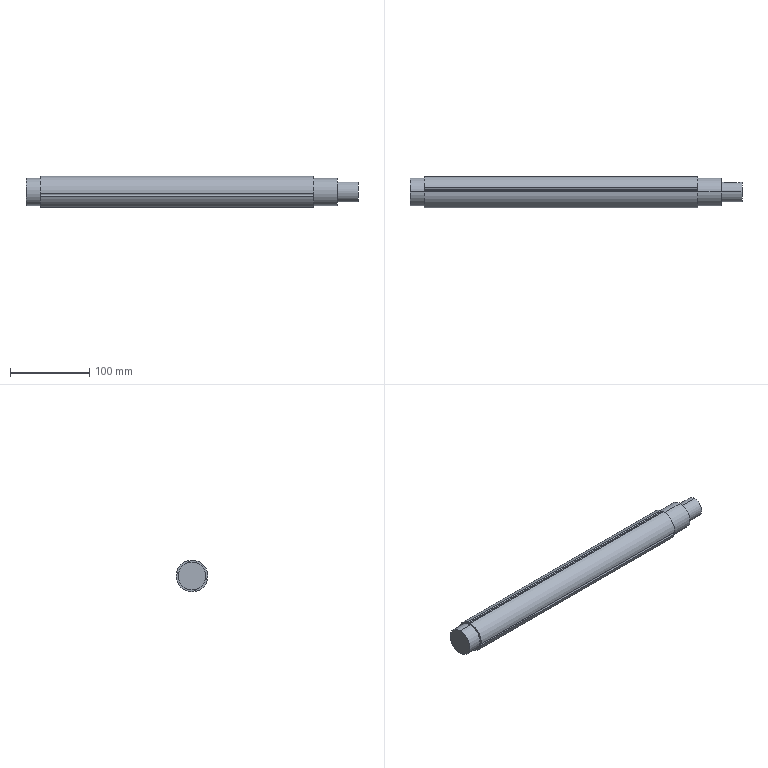Part | SolidWorks | features ICE 6, RefAxis 3, 3DProfileFeature 1, LockFeature 1, Revolution 1 | 1 solid | 26 faces | box 419 x 40 x 40 mm | volume 488497 mm3 | cylinder 18 | plane 8 | commonest cylinder face diameters 4.38 x5 40 x5 35 x4 8 x2 25 x2
STEP:
#1=CARTESIAN_POINT('',(193.5,11.843,-4.));
#2=VERTEX_POINT('',#1);
#3=CARTESIAN_POINT('',(193.5,11.843,4.));
#4=VERTEX_POINT('',#3);
#5=CARTESIAN_POINT('',(193.5,11.843,-4.));
#6=CARTESIAN_POINT('',(193.234,11.843,-4.));
#7=CARTESIAN_POINT('',(192.973,11.852,-3.974));
#8=CARTESIAN_POINT('',(192.459,11.886,-3.871));
#9=CARTESIAN_POINT('',(192.204,11.911,-3.793));
#10=CARTESIAN_POINT('',(191.721,11.973,-3.592));
#11=CARTESIAN_POINT('',(191.492,12.01,-3.469));
#12=CARTESIAN_POINT('',(191.059,12.09,-3.179));
#13=CARTESIAN_POINT('',(190.855,12.133,-3.012));
#14=CARTESIAN_POINT('',(190.489,12.218,-2.646));
#15=CARTESIAN_POINT('',(190.324,12.26,-2.445));
#16=CARTESIAN_POINT('',(190.031,12.34,-2.009));
#17=CARTESIAN_POINT('',(189.908,12.375,-1.779));
#18=CARTESIAN_POINT('',(189.708,12.435,-1.299));
#19=CARTESIAN_POINT('',(189.63,12.459,-1.045));
#20=CARTESIAN_POINT('',(189.526,12.492,-0.5276));
#21=CARTESIAN_POINT('',(189.5,12.5,-0.2669));
#22=CARTESIAN_POINT('',(189.5,12.5,0.2587));
#23=CARTESIAN_POINT('',(189.526,12.492,0.5256));
#24=CARTESIAN_POINT('',(189.629,12.459,1.04));
#25=CARTESIAN_POINT('',(189.705,12.436,1.29));
#26=CARTESIAN_POINT('',(189.907,12.375,1.777));
#27=CARTESIAN_POINT('',(190.031,12.34,2.008));
#28=CARTESIAN_POINT('',(190.32,12.262,2.44));
#29=CARTESIAN_POINT('',(190.487,12.219,2.643));
#30=CARTESIAN_POINT('',(190.855,12.133,3.012));
#31=CARTESIAN_POINT('',(191.055,12.091,3.176));
#32=CARTESIAN_POINT('',(191.487,12.011,3.466));
#33=CARTESIAN_POINT('',(191.72,11.973,3.592));
#34=CARTESIAN_POINT('',(192.202,11.911,3.792));
#35=CARTESIAN_POINT('',(192.451,11.886,3.869));
#36=CARTESIAN_POINT('',(192.968,11.852,3.973));
#37=CARTESIAN_POINT('',(193.234,11.843,4.));
#38=CARTESIAN_POINT('',(193.5,11.843,4.));
#39=B_SPLINE_CURVE_WITH_KNOTS('',3,(#5,#6,#7,#8,#9,#10,#11,#12,#13,#14,#15,#16,#17,#18,#19,#20,#21,#22,#23,#24,#25,#26,#27,#28,#29,#30,#31,#32,#33,#34,#35,#36,#37,#38),.UNSPECIFIED.,.F.,.F.,(4,2,2,2,2,2,2,2,2,2,2,2,2,2,2,2,4),(0.,0.0007865,0.001573,0.00236,0.003146,0.003933,0.004719,0.005506,0.006292,0.007079,0.007865,0.008652,0.009438,0.01022,0.01101,0.0118,0.01258),.UNSPECIFIED.);
#40=EDGE_CURVE('',#2,#4,#39,.T.);
#41=ORIENTED_EDGE('',*,*,#40,.F.);
#42=CARTESIAN_POINT('',(208.5,11.843,-4.));
#43=VERTEX_POINT('',#42);
#44=CARTESIAN_POINT('',(187.5,11.843,-4.));
#45=DIRECTION('',(-1.,0.,0.));
#46=VECTOR('',#45,1000.);
#47=LINE('',#44,#46);
#48=EDGE_CURVE('',#43,#2,#47,.T.);
#49=ORIENTED_EDGE('',*,*,#48,.F.);
#50=CARTESIAN_POINT('',(208.5,11.843,4.));
#51=VERTEX_POINT('',#50);
#52=CARTESIAN_POINT('',(208.5,11.843,4.));
#53=CARTESIAN_POINT('',(208.766,11.843,4.));
#54=CARTESIAN_POINT('',(209.027,11.852,3.974));
#55=CARTESIAN_POINT('',(209.541,11.886,3.871));
#56=CARTESIAN_POINT('',(209.796,11.911,3.793));
#57=CARTESIAN_POINT('',(210.279,11.973,3.592));
#58=CARTESIAN_POINT('',(210.508,12.01,3.469));
#59=CARTESIAN_POINT('',(210.941,12.09,3.179));
#60=CARTESIAN_POINT('',(211.145,12.133,3.012));
#61=CARTESIAN_POINT('',(211.511,12.218,2.646));
#62=CARTESIAN_POINT('',(211.676,12.26,2.445));
#63=CARTESIAN_POINT('',(211.969,12.34,2.009));
#64=CARTESIAN_POINT('',(212.092,12.375,1.779));
#65=CARTESIAN_POINT('',(212.292,12.435,1.299));
#66=CARTESIAN_POINT('',(212.37,12.459,1.045));
#67=CARTESIAN_POINT('',(212.474,12.492,0.5276));
#68=CARTESIAN_POINT('',(212.5,12.5,0.2669));
#69=CARTESIAN_POINT('',(212.5,12.5,-0.2587));
#70=CARTESIAN_POINT('',(212.474,12.492,-0.5256));
#71=CARTESIAN_POINT('',(212.371,12.459,-1.04));
#72=CARTESIAN_POINT('',(212.295,12.436,-1.29));
#73=CARTESIAN_POINT('',(212.093,12.375,-1.777));
#74=CARTESIAN_POINT('',(211.969,12.34,-2.008));
#75=CARTESIAN_POINT('',(211.68,12.262,-2.44));
#76=CARTESIAN_POINT('',(211.513,12.219,-2.643));
#77=CARTESIAN_POINT('',(211.145,12.133,-3.012));
#78=CARTESIAN_POINT('',(210.945,12.091,-3.176));
#79=CARTESIAN_POINT('',(210.513,12.011,-3.466));
#80=CARTESIAN_POINT('',(210.28,11.973,-3.592));
#81=CARTESIAN_POINT('',(209.798,11.911,-3.792));
#82=CARTESIAN_POINT('',(209.549,11.886,-3.869));
#83=CARTESIAN_POINT('',(209.032,11.852,-3.973));
#84=CARTESIAN_POINT('',(208.766,11.843,-4.));
#85=CARTESIAN_POINT('',(208.5,11.843,-4.));
#86=B_SPLINE_CURVE_WITH_KNOTS('',3,(#52,#53,#54,#55,#56,#57,#58,#59,#60,#61,#62,#63,#64,#65,#66,#67,#68,#69,#70,#71,#72,#73,#74,#75,#76,#77,#78,#79,#80,#81,#82,#83,#84,#85),.UNSPECIFIED.,.F.,.F.,(4,2,2,2,2,2,2,2,2,2,2,2,2,2,2,2,4),(0.,0.0007865,0.001573,0.00236,0.003146,0.003933,0.004719,0.005506,0.006292,0.007079,0.007865,0.008652,0.009438,0.01022,0.01101,0.0118,0.01258),.UNSPECIFIED.);
#87=EDGE_CURVE('',#51,#43,#86,.T.);
#88=ORIENTED_EDGE('',*,*,#87,.F.);
#89=CARTESIAN_POINT('',(187.5,11.843,4.));
#90=DIRECTION('',(1.,0.,0.));
#91=VECTOR('',#90,1000.);
#92=LINE('',#89,#91);
#93=EDGE_CURVE('',#4,#51,#92,.T.);
#94=ORIENTED_EDGE('',*,*,#93,.F.);
#95=EDGE_LOOP('',(#41,#49,#88,#94));
#96=FACE_BOUND('',#95,.T.);
#97=CARTESIAN_POINT('',(187.5,0.,-12.5));
#98=VERTEX_POINT('',#97);
#99=CARTESIAN_POINT('',(187.5,0.,12.5));
#100=VERTEX_POINT('',#99);
#101=CARTESIAN_POINT('',(187.5,0.,0.));
#102=DIRECTION('',(1.,0.,0.));
#103=DIRECTION('',(0.,0.,-1.));
#104=AXIS2_PLACEMENT_3D('',#101,#102,#103);
#105=CIRCLE('',#104,12.5);
#106=EDGE_CURVE('',#98,#100,#105,.T.);
#107=ORIENTED_EDGE('',*,*,#106,.T.);
#108=CARTESIAN_POINT('',(213.5,0.,12.5));
#109=VERTEX_POINT('',#108);
#110=CARTESIAN_POINT('',(187.5,0.,12.5));
#111=DIRECTION('',(1.,0.,0.));
#112=VECTOR('',#111,1000.);
#113=LINE('',#110,#112);
#114=EDGE_CURVE('',#100,#109,#113,.T.);
#115=ORIENTED_EDGE('',*,*,#114,.T.);
#116=CARTESIAN_POINT('',(213.5,0.,-12.5));
#117=VERTEX_POINT('',#116);
#118=CARTESIAN_POINT('',(213.5,0.,0.));
#119=DIRECTION('',(1.,0.,0.));
#120=DIRECTION('',(0.,0.,-1.));
#121=AXIS2_PLACEMENT_3D('',#118,#119,#120);
#122=CIRCLE('',#121,12.5);
#123=EDGE_CURVE('',#117,#109,#122,.T.);
#124=ORIENTED_EDGE('',*,*,#123,.F.);
#125=CARTESIAN_POINT('',(187.5,0.,-12.5));
#126=DIRECTION('',(1.,0.,0.));
#127=VECTOR('',#126,1000.);
#128=LINE('',#125,#127);
#129=EDGE_CURVE('',#98,#117,#128,.T.);
#130=ORIENTED_EDGE('',*,*,#129,.F.);
#131=EDGE_LOOP('',(#107,#115,#124,#130));
#132=FACE_OUTER_BOUND('',#131,.T.);
#133=CARTESIAN_POINT('',(187.5,0.,0.));
#134=DIRECTION('',(1.,0.,0.));
#135=DIRECTION('',(0.,0.,-1.));
#136=AXIS2_PLACEMENT_3D('',#133,#134,#135);
#137=CYLINDRICAL_SURFACE('',#136,12.5);
#138=ADVANCED_FACE('',(#96,#132),#137,.T.);
#139=CARTESIAN_POINT('',(157.5,0.,-17.5));
#140=VERTEX_POINT('',#139);
#141=CARTESIAN_POINT('',(157.5,0.,17.5));
#142=VERTEX_POINT('',#141);
#143=CARTESIAN_POINT('',(157.5,0.,0.));
#144=DIRECTION('',(1.,0.,0.));
#145=DIRECTION('',(0.,0.,-1.));
#146=AXIS2_PLACEMENT_3D('',#143,#144,#145);
#147=CIRCLE('',#146,17.5);
#148=EDGE_CURVE('',#140,#142,#147,.T.);
#149=ORIENTED_EDGE('',*,*,#148,.T.);
#150=CARTESIAN_POINT('',(187.5,0.,17.5));
#151=VERTEX_POINT('',#150);
#152=CARTESIAN_POINT('',(157.5,0.,17.5));
#153=DIRECTION('',(1.,0.,0.));
#154=VECTOR('',#153,1000.);
#155=LINE('',#152,#154);
#156=EDGE_CURVE('',#142,#151,#155,.T.);
#157=ORIENTED_EDGE('',*,*,#156,.T.);
#158=CARTESIAN_POINT('',(187.5,0.,-17.5));
#159=VERTEX_POINT('',#158);
#160=CARTESIAN_POINT('',(187.5,0.,0.));
#161=DIRECTION('',(1.,0.,0.));
#162=DIRECTION('',(0.,0.,-1.));
#163=AXIS2_PLACEMENT_3D('',#160,#161,#162);
#164=CIRCLE('',#163,17.5);
#165=EDGE_CURVE('',#159,#151,#164,.T.);
#166=ORIENTED_EDGE('',*,*,#165,.F.);
#167=CARTESIAN_POINT('',(157.5,0.,-17.5));
#168=DIRECTION('',(1.,0.,0.));
#169=VECTOR('',#168,1000.);
#170=LINE('',#167,#169);
#171=EDGE_CURVE('',#140,#159,#170,.T.);
#172=ORIENTED_EDGE('',*,*,#171,.F.);
#173=EDGE_LOOP('',(#149,#157,#166,#172));
#174=FACE_OUTER_BOUND('',#173,.T.);
#175=CARTESIAN_POINT('',(157.5,0.,0.));
#176=DIRECTION('',(1.,0.,0.));
#177=DIRECTION('',(0.,0.,-1.));
#178=AXIS2_PLACEMENT_3D('',#175,#176,#177);
#179=CYLINDRICAL_SURFACE('',#178,17.5);
#180=ADVANCED_FACE('',(#174),#179,.T.);
#181=CARTESIAN_POINT('',(-187.5,0.,17.5));
#182=VERTEX_POINT('',#181);
#183=CARTESIAN_POINT('',(-187.5,0.,-17.5));
#184=VERTEX_POINT('',#183);
#185=CARTESIAN_POINT('',(-187.5,0.,0.));
#186=DIRECTION('',(-1.,0.,0.));
#187=DIRECTION('',(0.,0.,1.));
#188=AXIS2_PLACEMENT_3D('',#185,#186,#187);
#189=CIRCLE('',#188,17.5);
#190=EDGE_CURVE('',#182,#184,#189,.T.);
#191=ORIENTED_EDGE('',*,*,#190,.T.);
#192=CARTESIAN_POINT('',(-205.5,0.,-17.5));
#193=VERTEX_POINT('',#192);
#194=CARTESIAN_POINT('',(-187.5,0.,-17.5));
#195=DIRECTION('',(-1.,0.,0.));
#196=VECTOR('',#195,1000.);
#197=LINE('',#194,#196);
#198=EDGE_CURVE('',#184,#193,#197,.T.);
#199=ORIENTED_EDGE('',*,*,#198,.T.);
#200=CARTESIAN_POINT('',(-205.5,0.,17.5));
#201=VERTEX_POINT('',#200);
#202=CARTESIAN_POINT('',(-205.5,0.,0.));
#203=DIRECTION('',(-1.,0.,0.));
#204=DIRECTION('',(0.,0.,1.));
#205=AXIS2_PLACEMENT_3D('',#202,#203,#204);
#206=CIRCLE('',#205,17.5);
#207=EDGE_CURVE('',#201,#193,#206,.T.);
#208=ORIENTED_EDGE('',*,*,#207,.F.);
#209=CARTESIAN_POINT('',(-187.5,0.,17.5));
#210=DIRECTION('',(-1.,0.,0.));
#211=VECTOR('',#210,1000.);
#212=LINE('',#209,#211);
#213=EDGE_CURVE('',#182,#201,#212,.T.);
#214=ORIENTED_EDGE('',*,*,#213,.F.);
#215=EDGE_LOOP('',(#191,#199,#208,#214));
#216=FACE_OUTER_BOUND('',#215,.T.);
#217=CARTESIAN_POINT('',(-187.5,0.,0.));
#218=DIRECTION('',(-1.,0.,0.));
#219=DIRECTION('',(0.,0.,1.));
#220=AXIS2_PLACEMENT_3D('',#217,#218,#219);
#221=CYLINDRICAL_SURFACE('',#220,17.5);
#222=ADVANCED_FACE('',(#216),#221,.T.);
#223=CARTESIAN_POINT('',(-187.5,5.203,19.311));
#224=VERTEX_POINT('',#223);
#225=CARTESIAN_POINT('',(-187.5,3.683,18.698));
#226=VERTEX_POINT('',#225);
#227=CARTESIAN_POINT('',(-187.5,3.683,20.888));
#228=DIRECTION('',(-1.,0.,0.));
#229=DIRECTION('',(0.,0.,1.));
#230=AXIS2_PLACEMENT_3D('',#227,#228,#229);
#231=CIRCLE('',#230,2.19);
#232=EDGE_CURVE('',#224,#226,#231,.T.);
#233=ORIENTED_EDGE('',*,*,#232,.T.);
#234=CARTESIAN_POINT('',(157.5,3.683,18.698));
#235=VERTEX_POINT('',#234);
#236=CARTESIAN_POINT('',(-205.5,3.683,18.698));
#237=DIRECTION('',(1.,0.,0.));
#238=VECTOR('',#237,1000.);
#239=LINE('',#236,#238);
#240=EDGE_CURVE('',#226,#235,#239,.T.);
#241=ORIENTED_EDGE('',*,*,#240,.T.);
#242=CARTESIAN_POINT('',(157.5,5.203,19.311));
#243=VERTEX_POINT('',#242);
#244=CARTESIAN_POINT('',(157.5,3.683,20.888));
#245=DIRECTION('',(1.,0.,0.));
#246=DIRECTION('',(0.,0.,-1.));
#247=AXIS2_PLACEMENT_3D('',#244,#245,#246);
#248=CIRCLE('',#247,2.19);
#249=EDGE_CURVE('',#235,#243,#248,.T.);
#250=ORIENTED_EDGE('',*,*,#249,.T.);
#251=CARTESIAN_POINT('',(-205.5,5.203,19.311));
#252=DIRECTION('',(1.,0.,0.));
#253=VECTOR('',#252,1000.);
#254=LINE('',#251,#253);
#255=EDGE_CURVE('',#224,#243,#254,.T.);
#256=ORIENTED_EDGE('',*,*,#255,.F.);
#257=EDGE_LOOP('',(#233,#241,#250,#256));
#258=FACE_OUTER_BOUND('',#257,.T.);
#259=CARTESIAN_POINT('',(-205.5,3.683,20.888));
#260=DIRECTION('',(1.,0.,0.));
#261=DIRECTION('',(0.,0.,-1.));
#262=AXIS2_PLACEMENT_3D('',#259,#260,#261);
#263=CYLINDRICAL_SURFACE('',#262,2.19);
#264=ADVANCED_FACE('',(#258),#263,.F.);
#265=CARTESIAN_POINT('',(157.5,0.,20.));
#266=VERTEX_POINT('',#265);
#267=CARTESIAN_POINT('',(157.5,-19.926,-1.715));
#268=VERTEX_POINT('',#267);
#269=CARTESIAN_POINT('',(157.5,0.,0.));
#270=DIRECTION('',(1.,0.,0.));
#271=DIRECTION('',(0.,0.,-1.));
#272=AXIS2_PLACEMENT_3D('',#269,#270,#271);
#273=CIRCLE('',#272,20.);
#274=EDGE_CURVE('',#266,#268,#273,.T.);
#275=ORIENTED_EDGE('',*,*,#274,.F.);
#276=CARTESIAN_POINT('',(-187.5,0.,20.));
#277=VERTEX_POINT('',#276);
#278=CARTESIAN_POINT('',(205.5,0.,20.));
#279=DIRECTION('',(-1.,0.,0.));
#280=VECTOR('',#279,1000.);
#281=LINE('',#278,#280);
#282=EDGE_CURVE('',#266,#277,#281,.T.);
#283=ORIENTED_EDGE('',*,*,#282,.T.);
#284=CARTESIAN_POINT('',(-187.5,-19.926,-1.715));
#285=VERTEX_POINT('',#284);
#286=CARTESIAN_POINT('',(-187.5,0.,0.));
#287=DIRECTION('',(-1.,0.,0.));
#288=DIRECTION('',(0.,0.,1.));
#289=AXIS2_PLACEMENT_3D('',#286,#287,#288);
#290=CIRCLE('',#289,20.);
#291=EDGE_CURVE('',#285,#277,#290,.T.);
#292=ORIENTED_EDGE('',*,*,#291,.F.);
#293=CARTESIAN_POINT('',(-205.5,-19.926,-1.715));
#294=DIRECTION('',(1.,0.,0.));
#295=VECTOR('',#294,1000.);
#296=LINE('',#293,#295);
#297=EDGE_CURVE('',#285,#268,#296,.T.);
#298=ORIENTED_EDGE('',*,*,#297,.T.);
#299=EDGE_LOOP('',(#275,#283,#292,#298));
#300=FACE_OUTER_BOUND('',#299,.T.);
#301=CARTESIAN_POINT('',(205.5,0.,0.));
#302=DIRECTION('',(-1.,0.,0.));
#303=DIRECTION('',(0.,0.,1.));
#304=AXIS2_PLACEMENT_3D('',#301,#302,#303);
#305=CYLINDRICAL_SURFACE('',#304,20.);
#306=ADVANCED_FACE('',(#300),#305,.T.);
#307=CARTESIAN_POINT('',(157.5,19.311,5.203));
#308=VERTEX_POINT('',#307);
#309=CARTESIAN_POINT('',(157.5,0.,0.));
#310=DIRECTION('',(1.,0.,0.));
#311=DIRECTION('',(0.,0.,-1.));
#312=AXIS2_PLACEMENT_3D('',#309,#310,#311);
#313=CIRCLE('',#312,20.);
#314=EDGE_CURVE('',#308,#243,#313,.T.);
#315=ORIENTED_EDGE('',*,*,#314,.F.);
#316=CARTESIAN_POINT('',(-187.5,19.311,5.203));
#317=VERTEX_POINT('',#316);
#318=CARTESIAN_POINT('',(-205.5,19.311,5.203));
#319=DIRECTION('',(1.,0.,0.));
#320=VECTOR('',#319,1000.);
#321=LINE('',#318,#320);
#322=EDGE_CURVE('',#317,#308,#321,.T.);
#323=ORIENTED_EDGE('',*,*,#322,.F.);
#324=CARTESIAN_POINT('',(-187.5,0.,0.));
#325=DIRECTION('',(-1.,0.,0.));
#326=DIRECTION('',(0.,0.,1.));
#327=AXIS2_PLACEMENT_3D('',#324,#325,#326);
#328=CIRCLE('',#327,20.);
#329=EDGE_CURVE('',#224,#317,#328,.T.);
#330=ORIENTED_EDGE('',*,*,#329,.F.);
#331=ORIENTED_EDGE('',*,*,#255,.T.);
#332=EDGE_LOOP('',(#315,#323,#330,#331));
#333=FACE_OUTER_BOUND('',#332,.T.);
#334=CARTESIAN_POINT('',(205.5,0.,0.));
#335=DIRECTION('',(-1.,0.,0.));
#336=DIRECTION('',(0.,0.,1.));
#337=AXIS2_PLACEMENT_3D('',#334,#335,#336);
#338=CYLINDRICAL_SURFACE('',#337,20.);
#339=ADVANCED_FACE('',(#333),#338,.T.);
#340=ORIENTED_EDGE('',*,*,#282,.F.);
#341=CARTESIAN_POINT('',(157.5,1.715,19.926));
#342=VERTEX_POINT('',#341);
#343=CARTESIAN_POINT('',(157.5,0.,0.));
#344=DIRECTION('',(1.,0.,0.));
#345=DIRECTION('',(0.,0.,-1.));
#346=AXIS2_PLACEMENT_3D('',#343,#344,#345);
#347=CIRCLE('',#346,20.);
#348=EDGE_CURVE('',#342,#266,#347,.T.);
#349=ORIENTED_EDGE('',*,*,#348,.F.);
#350=CARTESIAN_POINT('',(-187.5,1.715,19.926));
#351=VERTEX_POINT('',#350);
#352=CARTESIAN_POINT('',(-205.5,1.715,19.926));
#353=DIRECTION('',(1.,0.,0.));
#354=VECTOR('',#353,1000.);
#355=LINE('',#352,#354);
#356=EDGE_CURVE('',#351,#342,#355,.T.);
#357=ORIENTED_EDGE('',*,*,#356,.F.);
#358=CARTESIAN_POINT('',(-187.5,0.,0.));
#359=DIRECTION('',(-1.,0.,0.));
#360=DIRECTION('',(0.,0.,1.));
#361=AXIS2_PLACEMENT_3D('',#358,#359,#360);
#362=CIRCLE('',#361,20.);
#363=EDGE_CURVE('',#277,#351,#362,.T.);
#364=ORIENTED_EDGE('',*,*,#363,.F.);
#365=EDGE_LOOP('',(#340,#349,#357,#364));
#366=FACE_OUTER_BOUND('',#365,.T.);
#367=CARTESIAN_POINT('',(205.5,0.,0.));
#368=DIRECTION('',(-1.,0.,0.));
#369=DIRECTION('',(0.,0.,1.));
#370=AXIS2_PLACEMENT_3D('',#367,#368,#369);
#371=CYLINDRICAL_SURFACE('',#370,20.);
#372=ADVANCED_FACE('',(#366),#371,.T.);
#373=CARTESIAN_POINT('',(157.5,-1.715,-19.926));
#374=VERTEX_POINT('',#373);
#375=CARTESIAN_POINT('',(157.5,19.926,1.715));
#376=VERTEX_POINT('',#375);
#377=CARTESIAN_POINT('',(157.5,0.,0.));
#378=DIRECTION('',(1.,0.,0.));
#379=DIRECTION('',(0.,0.,-1.));
#380=AXIS2_PLACEMENT_3D('',#377,#378,#379);
#381=CIRCLE('',#380,20.);
#382=EDGE_CURVE('',#374,#376,#381,.T.);
#383=ORIENTED_EDGE('',*,*,#382,.F.);
#384=CARTESIAN_POINT('',(-187.5,-1.715,-19.926));
#385=VERTEX_POINT('',#384);
#386=CARTESIAN_POINT('',(-205.5,-1.715,-19.926));
#387=DIRECTION('',(1.,0.,0.));
#388=VECTOR('',#387,1000.);
#389=LINE('',#386,#388);
#390=EDGE_CURVE('',#385,#374,#389,.T.);
#391=ORIENTED_EDGE('',*,*,#390,.F.);
#392=CARTESIAN_POINT('',(-187.5,19.926,1.715));
#393=VERTEX_POINT('',#392);
#394=CARTESIAN_POINT('',(-187.5,0.,0.));
#395=DIRECTION('',(-1.,0.,0.));
#396=DIRECTION('',(0.,0.,1.));
#397=AXIS2_PLACEMENT_3D('',#394,#395,#396);
#398=CIRCLE('',#397,20.);
#399=EDGE_CURVE('',#393,#385,#398,.T.);
#400=ORIENTED_EDGE('',*,*,#399,.F.);
#401=CARTESIAN_POINT('',(-205.5,19.926,1.715));
#402=DIRECTION('',(1.,0.,0.));
#403=VECTOR('',#402,1000.);
#404=LINE('',#401,#403);
#405=EDGE_CURVE('',#393,#376,#404,.T.);
#406=ORIENTED_EDGE('',*,*,#405,.T.);
#407=EDGE_LOOP('',(#383,#391,#400,#406));
#408=FACE_OUTER_BOUND('',#407,.T.);
#409=CARTESIAN_POINT('',(205.5,0.,0.));
#410=DIRECTION('',(-1.,0.,0.));
#411=DIRECTION('',(0.,0.,1.));
#412=AXIS2_PLACEMENT_3D('',#409,#410,#411);
#413=CYLINDRICAL_SURFACE('',#412,20.);
#414=ADVANCED_FACE('',(#408),#413,.T.);
#415=CARTESIAN_POINT('',(157.5,-19.311,-5.203));
#416=VERTEX_POINT('',#415);
#417=CARTESIAN_POINT('',(157.5,-5.203,-19.311));
#418=VERTEX_POINT('',#417);
#419=CARTESIAN_POINT('',(157.5,0.,0.));
#420=DIRECTION('',(1.,0.,0.));
#421=DIRECTION('',(0.,0.,-1.));
#422=AXIS2_PLACEMENT_3D('',#419,#420,#421);
#423=CIRCLE('',#422,20.);
#424=EDGE_CURVE('',#416,#418,#423,.T.);
#425=ORIENTED_EDGE('',*,*,#424,.F.);
#426=CARTESIAN_POINT('',(-187.5,-19.311,-5.203));
#427=VERTEX_POINT('',#426);
#428=CARTESIAN_POINT('',(-205.5,-19.311,-5.203));
#429=DIRECTION('',(1.,0.,0.));
#430=VECTOR('',#429,1000.);
#431=LINE('',#428,#430);
#432=EDGE_CURVE('',#427,#416,#431,.T.);
#433=ORIENTED_EDGE('',*,*,#432,.F.);
#434=CARTESIAN_POINT('',(-187.5,-5.203,-19.311));
#435=VERTEX_POINT('',#434);
#436=CARTESIAN_POINT('',(-187.5,0.,0.));
#437=DIRECTION('',(-1.,0.,0.));
#438=DIRECTION('',(0.,0.,1.));
#439=AXIS2_PLACEMENT_3D('',#436,#437,#438);
#440=CIRCLE('',#439,20.);
#441=EDGE_CURVE('',#435,#427,#440,.T.);
#442=ORIENTED_EDGE('',*,*,#441,.F.);
#443=CARTESIAN_POINT('',(-205.5,-5.203,-19.311));
#444=DIRECTION('',(1.,0.,0.));
#445=VECTOR('',#444,1000.);
#446=LINE('',#443,#445);
#447=EDGE_CURVE('',#435,#418,#446,.T.);
#448=ORIENTED_EDGE('',*,*,#447,.T.);
#449=EDGE_LOOP('',(#425,#433,#442,#448));
#450=FACE_OUTER_BOUND('',#449,.T.);
#451=CARTESIAN_POINT('',(205.5,0.,0.));
#452=DIRECTION('',(-1.,0.,0.));
#453=DIRECTION('',(0.,0.,1.));
#454=AXIS2_PLACEMENT_3D('',#451,#452,#453);
#455=CYLINDRICAL_SURFACE('',#454,20.);
#456=ADVANCED_FACE('',(#450),#455,.T.);
#457=ORIENTED_EDGE('',*,*,#432,.T.);
#458=CARTESIAN_POINT('',(157.5,-20.888,-3.683));
#459=DIRECTION('',(1.,0.,0.));
#460=DIRECTION('',(0.,0.,-1.));
#461=AXIS2_PLACEMENT_3D('',#458,#459,#460);
#462=CIRCLE('',#461,2.19);
#463=EDGE_CURVE('',#416,#268,#462,.T.);
#464=ORIENTED_EDGE('',*,*,#463,.T.);
#465=ORIENTED_EDGE('',*,*,#297,.F.);
#466=CARTESIAN_POINT('',(-187.5,-20.888,-3.683));
#467=DIRECTION('',(-1.,0.,0.));
#468=DIRECTION('',(0.,0.,1.));
#469=AXIS2_PLACEMENT_3D('',#466,#467,#468);
#470=CIRCLE('',#469,2.19);
#471=EDGE_CURVE('',#285,#427,#470,.T.);
#472=ORIENTED_EDGE('',*,*,#471,.T.);
#473=EDGE_LOOP('',(#457,#464,#465,#472));
#474=FACE_OUTER_BOUND('',#473,.T.);
#475=CARTESIAN_POINT('',(-205.5,-20.888,-3.683));
#476=DIRECTION('',(1.,0.,0.));
#477=DIRECTION('',(0.,0.,-1.));
#478=AXIS2_PLACEMENT_3D('',#475,#476,#477);
#479=CYLINDRICAL_SURFACE('',#478,2.19);
#480=ADVANCED_FACE('',(#474),#479,.F.);
#481=ORIENTED_EDGE('',*,*,#390,.T.);
#482=CARTESIAN_POINT('',(157.5,-3.683,-20.888));
#483=DIRECTION('',(1.,0.,0.));
#484=DIRECTION('',(0.,0.,-1.));
#485=AXIS2_PLACEMENT_3D('',#482,#483,#484);
#486=CIRCLE('',#485,2.19);
#487=EDGE_CURVE('',#374,#418,#486,.T.);
#488=ORIENTED_EDGE('',*,*,#487,.T.);
#489=ORIENTED_EDGE('',*,*,#447,.F.);
#490=CARTESIAN_POINT('',(-187.5,-3.683,-20.888));
#491=DIRECTION('',(-1.,0.,0.));
#492=DIRECTION('',(0.,0.,1.));
#493=AXIS2_PLACEMENT_3D('',#490,#491,#492);
#494=CIRCLE('',#493,2.19);
#495=EDGE_CURVE('',#435,#385,#494,.T.);
#496=ORIENTED_EDGE('',*,*,#495,.T.);
#497=EDGE_LOOP('',(#481,#488,#489,#496));
#498=FACE_OUTER_BOUND('',#497,.T.);
#499=CARTESIAN_POINT('',(-205.5,-3.683,-20.888));
#500=DIRECTION('',(1.,0.,0.));
#501=DIRECTION('',(0.,0.,-1.));
#502=AXIS2_PLACEMENT_3D('',#499,#500,#501);
#503=CYLINDRICAL_SURFACE('',#502,2.19);
#504=ADVANCED_FACE('',(#498),#503,.F.);
#505=ORIENTED_EDGE('',*,*,#322,.T.);
#506=CARTESIAN_POINT('',(157.5,20.888,3.683));
#507=DIRECTION('',(1.,0.,0.));
#508=DIRECTION('',(0.,0.,-1.));
#509=AXIS2_PLACEMENT_3D('',#506,#507,#508);
#510=CIRCLE('',#509,2.19);
#511=EDGE_CURVE('',#308,#376,#510,.T.);
#512=ORIENTED_EDGE('',*,*,#511,.T.);
#513=ORIENTED_EDGE('',*,*,#405,.F.);
#514=CARTESIAN_POINT('',(-187.5,20.888,3.683));
#515=DIRECTION('',(-1.,0.,0.));
#516=DIRECTION('',(0.,0.,1.));
#517=AXIS2_PLACEMENT_3D('',#514,#515,#516);
#518=CIRCLE('',#517,2.19);
#519=EDGE_CURVE('',#393,#317,#518,.T.);
#520=ORIENTED_EDGE('',*,*,#519,.T.);
#521=EDGE_LOOP('',(#505,#512,#513,#520));
#522=FACE_OUTER_BOUND('',#521,.T.);
#523=CARTESIAN_POINT('',(-205.5,20.888,3.683));
#524=DIRECTION('',(1.,0.,0.));
#525=DIRECTION('',(0.,0.,-1.));
#526=AXIS2_PLACEMENT_3D('',#523,#524,#525);
#527=CYLINDRICAL_SURFACE('',#526,2.19);
#528=ADVANCED_FACE('',(#522),#527,.F.);
#529=ORIENTED_EDGE('',*,*,#240,.F.);
#530=CARTESIAN_POINT('',(-187.5,3.683,20.888));
#531=DIRECTION('',(-1.,0.,0.));
#532=DIRECTION('',(0.,0.,1.));
#533=AXIS2_PLACEMENT_3D('',#530,#531,#532);
#534=CIRCLE('',#533,2.19);
#535=EDGE_CURVE('',#226,#351,#534,.T.);
#536=ORIENTED_EDGE('',*,*,#535,.T.);
#537=ORIENTED_EDGE('',*,*,#356,.T.);
#538=CARTESIAN_POINT('',(157.5,3.683,20.888));
#539=DIRECTION('',(1.,0.,0.));
#540=DIRECTION('',(0.,0.,-1.));
#541=AXIS2_PLACEMENT_3D('',#538,#539,#540);
#542=CIRCLE('',#541,2.19);
#543=EDGE_CURVE('',#342,#235,#542,.T.);
#544=ORIENTED_EDGE('',*,*,#543,.T.);
#545=EDGE_LOOP('',(#529,#536,#537,#544));
#546=FACE_OUTER_BOUND('',#545,.T.);
#547=CARTESIAN_POINT('',(-205.5,3.683,20.888));
#548=DIRECTION('',(1.,0.,0.));
#549=DIRECTION('',(0.,0.,-1.));
#550=AXIS2_PLACEMENT_3D('',#547,#548,#549);
#551=CYLINDRICAL_SURFACE('',#550,2.19);
#552=ADVANCED_FACE('',(#546),#551,.F.);
#553=ORIENTED_EDGE('',*,*,#441,.T.);
#554=ORIENTED_EDGE('',*,*,#471,.F.);
#555=ORIENTED_EDGE('',*,*,#291,.T.);
#556=ORIENTED_EDGE('',*,*,#363,.T.);
#557=ORIENTED_EDGE('',*,*,#535,.F.);
#558=ORIENTED_EDGE('',*,*,#232,.F.);
#559=ORIENTED_EDGE('',*,*,#329,.T.);
#560=ORIENTED_EDGE('',*,*,#519,.F.);
#561=ORIENTED_EDGE('',*,*,#399,.T.);
#562=ORIENTED_EDGE('',*,*,#495,.F.);
#563=EDGE_LOOP('',(#553,#554,#555,#556,#557,#558,#559,#560,#561,#562));
#564=FACE_OUTER_BOUND('',#563,.T.);
#565=ORIENTED_EDGE('',*,*,#190,.F.);
#566=CARTESIAN_POINT('',(-187.5,0.,0.));
#567=DIRECTION('',(-1.,0.,0.));
#568=DIRECTION('',(0.,0.,1.));
#569=AXIS2_PLACEMENT_3D('',#566,#567,#568);
#570=CIRCLE('',#569,17.5);
#571=EDGE_CURVE('',#184,#182,#570,.T.);
#572=ORIENTED_EDGE('',*,*,#571,.F.);
#573=EDGE_LOOP('',(#565,#572));
#574=FACE_BOUND('',#573,.T.);
#575=CARTESIAN_POINT('',(-187.5,0.,0.));
#576=DIRECTION('',(-1.,0.,0.));
#577=DIRECTION('',(0.,0.,1.));
#578=AXIS2_PLACEMENT_3D('',#575,#576,#577);
#579=PLANE('',#578);
#580=ADVANCED_FACE('',(#564,#574),#579,.T.);
#581=ORIENTED_EDGE('',*,*,#198,.F.);
#582=ORIENTED_EDGE('',*,*,#571,.T.);
#583=ORIENTED_EDGE('',*,*,#213,.T.);
#584=CARTESIAN_POINT('',(-205.5,0.,0.));
#585=DIRECTION('',(-1.,0.,0.));
#586=DIRECTION('',(0.,0.,1.));
#587=AXIS2_PLACEMENT_3D('',#584,#585,#586);
#588=CIRCLE('',#587,17.5);
#589=EDGE_CURVE('',#193,#201,#588,.T.);
#590=ORIENTED_EDGE('',*,*,#589,.F.);
#591=EDGE_LOOP('',(#581,#582,#583,#590));
#592=FACE_OUTER_BOUND('',#591,.T.);
#593=CARTESIAN_POINT('',(-187.5,0.,0.));
#594=DIRECTION('',(-1.,0.,0.));
#595=DIRECTION('',(0.,0.,1.));
#596=AXIS2_PLACEMENT_3D('',#593,#594,#595);
#597=CYLINDRICAL_SURFACE('',#596,17.5);
#598=ADVANCED_FACE('',(#592),#597,.T.);
#599=ORIENTED_EDGE('',*,*,#207,.T.);
#600=ORIENTED_EDGE('',*,*,#589,.T.);
#601=EDGE_LOOP('',(#599,#600));
#602=FACE_OUTER_BOUND('',#601,.T.);
#603=CARTESIAN_POINT('',(-205.5,0.,0.));
#604=DIRECTION('',(1.,0.,0.));
#605=DIRECTION('',(0.,0.,-1.));
#606=AXIS2_PLACEMENT_3D('',#603,#604,#605);
#607=PLANE('',#606);
#608=ADVANCED_FACE('',(#602),#607,.F.);
#609=ORIENTED_EDGE('',*,*,#382,.T.);
#610=ORIENTED_EDGE('',*,*,#511,.F.);
#611=ORIENTED_EDGE('',*,*,#314,.T.);
#612=ORIENTED_EDGE('',*,*,#249,.F.);
#613=ORIENTED_EDGE('',*,*,#543,.F.);
#614=ORIENTED_EDGE('',*,*,#348,.T.);
#615=ORIENTED_EDGE('',*,*,#274,.T.);
#616=ORIENTED_EDGE('',*,*,#463,.F.);
#617=ORIENTED_EDGE('',*,*,#424,.T.);
#618=ORIENTED_EDGE('',*,*,#487,.F.);
#619=EDGE_LOOP('',(#609,#610,#611,#612,#613,#614,#615,#616,#617,#618));
#620=FACE_OUTER_BOUND('',#619,.T.);
#621=ORIENTED_EDGE('',*,*,#148,.F.);
#622=CARTESIAN_POINT('',(157.5,0.,0.));
#623=DIRECTION('',(1.,0.,0.));
#624=DIRECTION('',(0.,0.,-1.));
#625=AXIS2_PLACEMENT_3D('',#622,#623,#624);
#626=CIRCLE('',#625,17.5);
#627=EDGE_CURVE('',#142,#140,#626,.T.);
#628=ORIENTED_EDGE('',*,*,#627,.F.);
#629=EDGE_LOOP('',(#621,#628));
#630=FACE_BOUND('',#629,.T.);
#631=CARTESIAN_POINT('',(157.5,0.,0.));
#632=DIRECTION('',(1.,0.,0.));
#633=DIRECTION('',(0.,0.,-1.));
#634=AXIS2_PLACEMENT_3D('',#631,#632,#633);
#635=PLANE('',#634);
#636=ADVANCED_FACE('',(#620,#630),#635,.T.);
#637=ORIENTED_EDGE('',*,*,#156,.F.);
#638=ORIENTED_EDGE('',*,*,#627,.T.);
#639=ORIENTED_EDGE('',*,*,#171,.T.);
#640=CARTESIAN_POINT('',(187.5,0.,0.));
#641=DIRECTION('',(1.,0.,0.));
#642=DIRECTION('',(0.,0.,-1.));
#643=AXIS2_PLACEMENT_3D('',#640,#641,#642);
#644=CIRCLE('',#643,17.5);
#645=EDGE_CURVE('',#151,#159,#644,.T.);
#646=ORIENTED_EDGE('',*,*,#645,.F.);
#647=EDGE_LOOP('',(#637,#638,#639,#646));
#648=FACE_OUTER_BOUND('',#647,.T.);
#649=CARTESIAN_POINT('',(157.5,0.,0.));
#650=DIRECTION('',(1.,0.,0.));
#651=DIRECTION('',(0.,0.,-1.));
#652=AXIS2_PLACEMENT_3D('',#649,#650,#651);
#653=CYLINDRICAL_SURFACE('',#652,17.5);
#654=ADVANCED_FACE('',(#648),#653,.T.);
#655=ORIENTED_EDGE('',*,*,#114,.F.);
#656=CARTESIAN_POINT('',(187.5,0.,0.));
#657=DIRECTION('',(1.,0.,0.));
#658=DIRECTION('',(0.,0.,-1.));
#659=AXIS2_PLACEMENT_3D('',#656,#657,#658);
#660=CIRCLE('',#659,12.5);
#661=EDGE_CURVE('',#100,#98,#660,.T.);
#662=ORIENTED_EDGE('',*,*,#661,.T.);
#663=ORIENTED_EDGE('',*,*,#129,.T.);
#664=CARTESIAN_POINT('',(213.5,0.,0.));
#665=DIRECTION('',(1.,0.,0.));
#666=DIRECTION('',(0.,0.,-1.));
#667=AXIS2_PLACEMENT_3D('',#664,#665,#666);
#668=CIRCLE('',#667,12.5);
#669=EDGE_CURVE('',#109,#117,#668,.T.);
#670=ORIENTED_EDGE('',*,*,#669,.F.);
#671=EDGE_LOOP('',(#655,#662,#663,#670));
#672=FACE_OUTER_BOUND('',#671,.T.);
#673=CARTESIAN_POINT('',(187.5,0.,0.));
#674=DIRECTION('',(1.,0.,0.));
#675=DIRECTION('',(0.,0.,-1.));
#676=AXIS2_PLACEMENT_3D('',#673,#674,#675);
#677=CYLINDRICAL_SURFACE('',#676,12.5);
#678=ADVANCED_FACE('',(#672),#677,.T.);
#679=ORIENTED_EDGE('',*,*,#106,.F.);
#680=ORIENTED_EDGE('',*,*,#661,.F.);
#681=EDGE_LOOP('',(#679,#680));
#682=FACE_BOUND('',#681,.T.);
#683=ORIENTED_EDGE('',*,*,#165,.T.);
#684=ORIENTED_EDGE('',*,*,#645,.T.);
#685=EDGE_LOOP('',(#683,#684));
#686=FACE_OUTER_BOUND('',#685,.T.);
#687=CARTESIAN_POINT('',(187.5,0.,0.));
#688=DIRECTION('',(1.,0.,0.));
#689=DIRECTION('',(0.,0.,-1.));
#690=AXIS2_PLACEMENT_3D('',#687,#688,#689);
#691=PLANE('',#690);
#692=ADVANCED_FACE('',(#682,#686),#691,.T.);
#693=ORIENTED_EDGE('',*,*,#123,.T.);
#694=ORIENTED_EDGE('',*,*,#669,.T.);
#695=EDGE_LOOP('',(#693,#694));
#696=FACE_OUTER_BOUND('',#695,.T.);
#697=CARTESIAN_POINT('',(213.5,0.,0.));
#698=DIRECTION('',(1.,0.,0.));
#699=DIRECTION('',(0.,0.,-1.));
#700=AXIS2_PLACEMENT_3D('',#697,#698,#699);
#701=PLANE('',#700);
#702=ADVANCED_FACE('',(#696),#701,.T.);
#703=CARTESIAN_POINT('',(208.5,8.5,4.));
#704=VERTEX_POINT('',#703);
#705=CARTESIAN_POINT('',(208.5,8.5,4.));
#706=DIRECTION('',(0.,1.,0.));
#707=VECTOR('',#706,1000.);
#708=LINE('',#705,#707);
#709=EDGE_CURVE('',#704,#51,#708,.T.);
#710=ORIENTED_EDGE('',*,*,#709,.T.);
#711=ORIENTED_EDGE('',*,*,#87,.T.);
#712=CARTESIAN_POINT('',(208.5,8.5,-4.));
#713=VERTEX_POINT('',#712);
#714=CARTESIAN_POINT('',(208.5,8.5,-4.));
#715=DIRECTION('',(0.,1.,0.));
#716=VECTOR('',#715,1000.);
#717=LINE('',#714,#716);
#718=EDGE_CURVE('',#713,#43,#717,.T.);
#719=ORIENTED_EDGE('',*,*,#718,.F.);
#720=CARTESIAN_POINT('',(208.5,8.5,0.));
#721=DIRECTION('',(0.,1.,0.));
#722=DIRECTION('',(0.,0.,1.));
#723=AXIS2_PLACEMENT_3D('',#720,#721,#722);
#724=CIRCLE('',#723,4.);
#725=EDGE_CURVE('',#704,#713,#724,.T.);
#726=ORIENTED_EDGE('',*,*,#725,.F.);
#727=EDGE_LOOP('',(#710,#711,#719,#726));
#728=FACE_OUTER_BOUND('',#727,.T.);
#729=CARTESIAN_POINT('',(208.5,8.5,0.));
#730=DIRECTION('',(0.,1.,0.));
#731=DIRECTION('',(0.,0.,1.));
#732=AXIS2_PLACEMENT_3D('',#729,#730,#731);
#733=CYLINDRICAL_SURFACE('',#732,4.);
#734=ADVANCED_FACE('',(#728),#733,.F.);
#735=ORIENTED_EDGE('',*,*,#93,.T.);
#736=ORIENTED_EDGE('',*,*,#709,.F.);
#737=CARTESIAN_POINT('',(193.5,8.5,4.));
#738=VERTEX_POINT('',#737);
#739=CARTESIAN_POINT('',(208.5,8.5,4.));
#740=DIRECTION('',(1.,0.,0.));
#741=VECTOR('',#740,1000.);
#742=LINE('',#739,#741);
#743=EDGE_CURVE('',#738,#704,#742,.T.);
#744=ORIENTED_EDGE('',*,*,#743,.F.);
#745=CARTESIAN_POINT('',(193.5,8.5,4.));
#746=DIRECTION('',(0.,1.,0.));
#747=VECTOR('',#746,1000.);
#748=LINE('',#745,#747);
#749=EDGE_CURVE('',#738,#4,#748,.T.);
#750=ORIENTED_EDGE('',*,*,#749,.T.);
#751=EDGE_LOOP('',(#735,#736,#744,#750));
#752=FACE_OUTER_BOUND('',#751,.T.);
#753=CARTESIAN_POINT('',(208.5,8.5,4.));
#754=DIRECTION('',(0.,0.,1.));
#755=DIRECTION('',(1.,0.,0.));
#756=AXIS2_PLACEMENT_3D('',#753,#754,#755);
#757=PLANE('',#756);
#758=ADVANCED_FACE('',(#752),#757,.F.);
#759=CARTESIAN_POINT('',(193.5,8.5,-4.));
#760=VERTEX_POINT('',#759);
#761=CARTESIAN_POINT('',(193.5,8.5,-4.));
#762=DIRECTION('',(0.,1.,0.));
#763=VECTOR('',#762,1000.);
#764=LINE('',#761,#763);
#765=EDGE_CURVE('',#760,#2,#764,.T.);
#766=ORIENTED_EDGE('',*,*,#765,.T.);
#767=ORIENTED_EDGE('',*,*,#40,.T.);
#768=ORIENTED_EDGE('',*,*,#749,.F.);
#769=CARTESIAN_POINT('',(193.5,8.5,0.));
#770=DIRECTION('',(0.,1.,0.));
#771=DIRECTION('',(0.,0.,1.));
#772=AXIS2_PLACEMENT_3D('',#769,#770,#771);
#773=CIRCLE('',#772,4.);
#774=EDGE_CURVE('',#760,#738,#773,.T.);
#775=ORIENTED_EDGE('',*,*,#774,.F.);
#776=EDGE_LOOP('',(#766,#767,#768,#775));
#777=FACE_OUTER_BOUND('',#776,.T.);
#778=CARTESIAN_POINT('',(193.5,8.5,0.));
#779=DIRECTION('',(0.,1.,0.));
#780=DIRECTION('',(0.,0.,1.));
#781=AXIS2_PLACEMENT_3D('',#778,#779,#780);
#782=CYLINDRICAL_SURFACE('',#781,4.);
#783=ADVANCED_FACE('',(#777),#782,.F.);
#784=ORIENTED_EDGE('',*,*,#48,.T.);
#785=ORIENTED_EDGE('',*,*,#765,.F.);
#786=CARTESIAN_POINT('',(208.5,8.5,-4.));
#787=DIRECTION('',(-1.,0.,0.));
#788=VECTOR('',#787,1000.);
#789=LINE('',#786,#788);
#790=EDGE_CURVE('',#713,#760,#789,.T.);
#791=ORIENTED_EDGE('',*,*,#790,.F.);
#792=ORIENTED_EDGE('',*,*,#718,.T.);
#793=EDGE_LOOP('',(#784,#785,#791,#792));
#794=FACE_OUTER_BOUND('',#793,.T.);
#795=CARTESIAN_POINT('',(208.5,8.5,-4.));
#796=DIRECTION('',(0.,0.,-1.));
#797=DIRECTION('',(-1.,0.,0.));
#798=AXIS2_PLACEMENT_3D('',#795,#796,#797);
#799=PLANE('',#798);
#800=ADVANCED_FACE('',(#794),#799,.F.);
#801=ORIENTED_EDGE('',*,*,#725,.T.);
#802=ORIENTED_EDGE('',*,*,#790,.T.);
#803=ORIENTED_EDGE('',*,*,#774,.T.);
#804=ORIENTED_EDGE('',*,*,#743,.T.);
#805=EDGE_LOOP('',(#801,#802,#803,#804));
#806=FACE_OUTER_BOUND('',#805,.T.);
#807=CARTESIAN_POINT('',(208.5,8.5,0.));
#808=DIRECTION('',(0.,1.,0.));
#809=DIRECTION('',(0.,0.,1.));
#810=AXIS2_PLACEMENT_3D('',#807,#808,#809);
#811=PLANE('',#810);
#812=ADVANCED_FACE('',(#806),#811,.T.);
#813=CLOSED_SHELL('',(#138,#180,#222,#264,#306,#339,#372,#414,#456,#480,#504,#528,#552,#580,#598,#608,#636,#654,#678,#692,#702,#734,#758,#783,#800,#812));
#814=MANIFOLD_SOLID_BREP('',#813);
#815=CARTESIAN_POINT('',(0.,0.,0.));
#816=DIRECTION('',(0.,0.,1.));
#817=DIRECTION('',(1.,0.,0.));
#818=AXIS2_PLACEMENT_3D('',#815,#816,#817);
#819=(LENGTH_UNIT()NAMED_UNIT(*)SI_UNIT(.MILLI.,.METRE.));
#820=UNCERTAINTY_MEASURE_WITH_UNIT(LENGTH_MEASURE(0.00001),#819,'','');
#821=(NAMED_UNIT(*)PLANE_ANGLE_UNIT()SI_UNIT($,.RADIAN.));
#822=(NAMED_UNIT(*)SI_UNIT($,.STERADIAN.)SOLID_ANGLE_UNIT());
#823=(GEOMETRIC_REPRESENTATION_CONTEXT(3)GLOBAL_UNCERTAINTY_ASSIGNED_CONTEXT((#820))GLOBAL_UNIT_ASSIGNED_CONTEXT((#819,#821,#822))REPRESENTATION_CONTEXT('',''));
#824=ADVANCED_BREP_SHAPE_REPRESENTATION('',(#814,#818),#823);